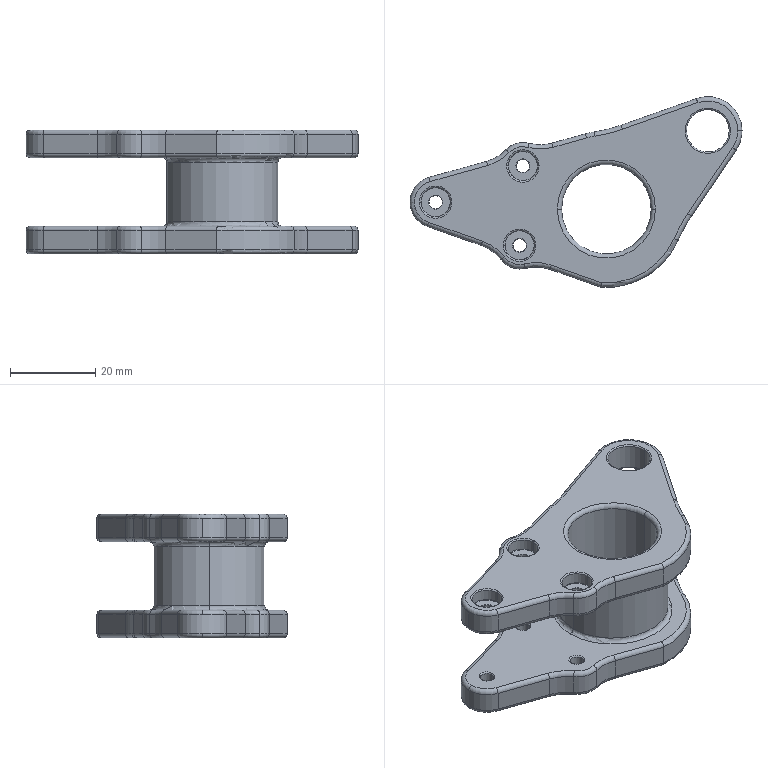Part | SolidWorks | features ICE 7, Fillet 6, Extrusion 1, MirrorPattern 1 | 1 solid | 220 faces | box 77.714 x 44.619 x 29 mm | volume 22578 mm3 | torus 116 | cylinder 82 | plane 22 | commonest cylinder face diameters 2 x24 3.1 x12 7 x12 20 x8 10 x4 11 x4